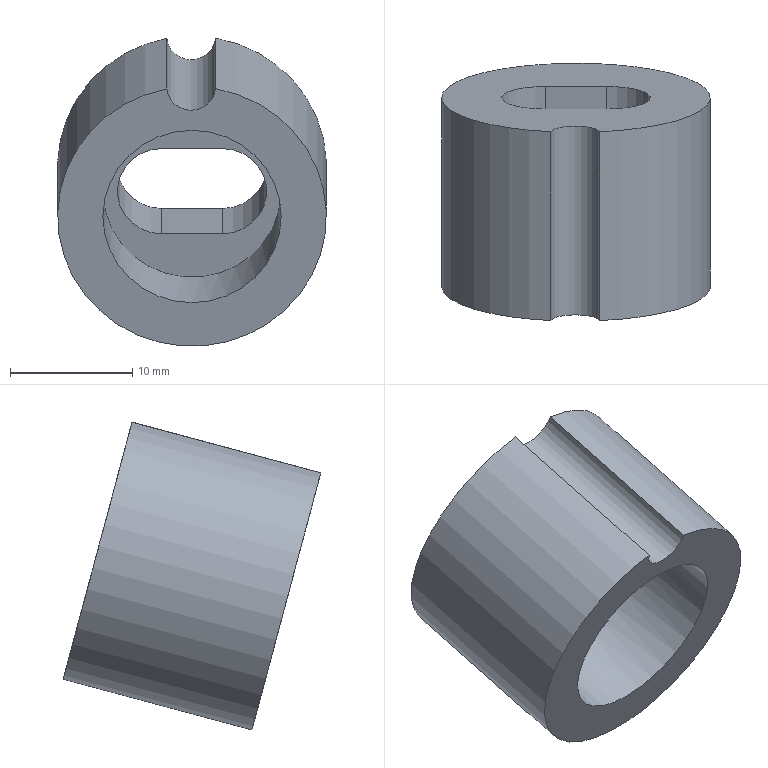Part | NX | features solid 2 | 1 solid | 10 faces | box 22 x 21.105 x 25.227 mm | volume 4030 mm3 | plane 5 | cylinder 5 | commonest cylinder face diameters 7.22 x2 4 x1 14.6 x1 22 x1
STEP:
#1=CARTESIAN_POINT('',(-406.307,59.873,-23.154));
#2=VERTEX_POINT('',#1);
#3=CARTESIAN_POINT('',(-402.324,59.867,-23.131));
#4=VERTEX_POINT('',#3);
#5=CARTESIAN_POINT('',(-404.316,59.823,-22.965));
#6=DIRECTION('',(0.,-0.9659,-0.2588));
#7=DIRECTION('',(0.999,0.01147,-0.04282));
#8=AXIS2_PLACEMENT_3D('',#5,#6,#7);
#9=CIRCLE('',#8,2.);
#10=EDGE_CURVE('',#2,#4,#9,.T.);
#11=ORIENTED_EDGE('',*,*,#10,.T.);
#12=CARTESIAN_POINT('',(-404.25,62.67,-33.592));
#13=DIRECTION('',(0.,0.9659,0.2588));
#14=DIRECTION('',(0.,-0.2588,0.9659));
#15=AXIS2_PLACEMENT_3D('',#12,#13,#14);
#16=CIRCLE('',#15,11.);
#17=EDGE_CURVE('',#2,#4,#16,.F.);
#18=ORIENTED_EDGE('',*,*,#17,.F.);
#19=EDGE_LOOP('',(#11,#18));
#20=FACE_BOUND('',#19,.T.);
#21=CARTESIAN_POINT('',(-401.75,63.604,-37.079));
#22=VERTEX_POINT('',#21);
#23=CARTESIAN_POINT('',(-401.75,61.736,-30.105));
#24=VERTEX_POINT('',#23);
#25=CARTESIAN_POINT('',(-401.75,62.67,-33.592));
#26=DIRECTION('',(0.,0.9659,0.2588));
#27=DIRECTION('',(0.,-0.2588,0.9659));
#28=AXIS2_PLACEMENT_3D('',#25,#26,#27);
#29=CIRCLE('',#28,3.61);
#30=EDGE_CURVE('',#22,#24,#29,.F.);
#31=ORIENTED_EDGE('',*,*,#30,.T.);
#32=CARTESIAN_POINT('',(-406.75,61.736,-30.105));
#33=VERTEX_POINT('',#32);
#34=CARTESIAN_POINT('',(-404.25,61.736,-30.105));
#35=DIRECTION('',(-1.,0.,0.));
#36=VECTOR('',#35,1000.);
#37=LINE('',#34,#36);
#38=EDGE_CURVE('',#24,#33,#37,.T.);
#39=ORIENTED_EDGE('',*,*,#38,.T.);
#40=CARTESIAN_POINT('',(-406.75,63.604,-37.079));
#41=VERTEX_POINT('',#40);
#42=CARTESIAN_POINT('',(-406.75,62.67,-33.592));
#43=DIRECTION('',(0.,0.9659,0.2588));
#44=DIRECTION('',(0.,-0.2588,0.9659));
#45=AXIS2_PLACEMENT_3D('',#42,#43,#44);
#46=CIRCLE('',#45,3.61);
#47=EDGE_CURVE('',#33,#41,#46,.F.);
#48=ORIENTED_EDGE('',*,*,#47,.T.);
#49=CARTESIAN_POINT('',(-404.25,63.604,-37.079));
#50=DIRECTION('',(1.,0.,0.));
#51=VECTOR('',#50,1000.);
#52=LINE('',#49,#51);
#53=EDGE_CURVE('',#41,#22,#52,.T.);
#54=ORIENTED_EDGE('',*,*,#53,.T.);
#55=EDGE_LOOP('',(#31,#39,#48,#54));
#56=FACE_BOUND('',#55,.T.);
#57=CARTESIAN_POINT('',(-404.25,62.67,-33.592));
#58=DIRECTION('',(0.,0.9659,0.2588));
#59=DIRECTION('',(-0.999,-0.01147,0.04282));
#60=AXIS2_PLACEMENT_3D('',#57,#58,#59);
#61=PLANE('',#60);
#62=ADVANCED_FACE('',(#20,#56),#61,.T.);
#63=CARTESIAN_POINT('',(-402.324,44.412,-27.272));
#64=VERTEX_POINT('',#63);
#65=CARTESIAN_POINT('',(-406.307,44.418,-27.295));
#66=VERTEX_POINT('',#65);
#67=CARTESIAN_POINT('',(-404.316,44.368,-27.106));
#68=DIRECTION('',(0.,-0.9659,-0.2588));
#69=DIRECTION('',(0.,0.2588,-0.9659));
#70=AXIS2_PLACEMENT_3D('',#67,#68,#69);
#71=CIRCLE('',#70,2.);
#72=EDGE_CURVE('',#64,#66,#71,.F.);
#73=ORIENTED_EDGE('',*,*,#72,.T.);
#74=CARTESIAN_POINT('',(-404.25,47.215,-37.733));
#75=DIRECTION('',(0.,-0.9659,-0.2588));
#76=DIRECTION('',(0.,0.2588,-0.9659));
#77=AXIS2_PLACEMENT_3D('',#74,#75,#76);
#78=CIRCLE('',#77,11.);
#79=EDGE_CURVE('',#64,#66,#78,.F.);
#80=ORIENTED_EDGE('',*,*,#79,.F.);
#81=EDGE_LOOP('',(#73,#80));
#82=FACE_BOUND('',#81,.T.);
#83=CARTESIAN_POINT('',(-404.25,49.105,-44.784));
#84=VERTEX_POINT('',#83);
#85=CARTESIAN_POINT('',(-404.25,47.215,-37.733));
#86=DIRECTION('',(0.,-0.9659,-0.2588));
#87=DIRECTION('',(0.,0.2588,-0.9659));
#88=AXIS2_PLACEMENT_3D('',#85,#86,#87);
#89=CIRCLE('',#88,7.3);
#90=EDGE_CURVE('',#84,#84,#89,.F.);
#91=ORIENTED_EDGE('',*,*,#90,.T.);
#92=EDGE_LOOP('',(#91));
#93=FACE_BOUND('',#92,.T.);
#94=CARTESIAN_POINT('',(-404.25,47.215,-37.733));
#95=DIRECTION('',(0.,-0.9659,-0.2588));
#96=DIRECTION('',(0.999,0.01147,-0.04282));
#97=AXIS2_PLACEMENT_3D('',#94,#95,#96);
#98=PLANE('',#97);
#99=ADVANCED_FACE('',(#82,#93),#98,.T.);
#100=CARTESIAN_POINT('',(-402.324,52.14,-25.201));
#101=DIRECTION('',(0.,0.9659,0.2588));
#102=VECTOR('',#101,1000.);
#103=LINE('',#100,#102);
#104=EDGE_CURVE('',#64,#4,#103,.T.);
#105=ORIENTED_EDGE('',*,*,#104,.F.);
#106=ORIENTED_EDGE('',*,*,#79,.T.);
#107=CARTESIAN_POINT('',(-406.307,52.146,-25.225));
#108=DIRECTION('',(0.,0.9659,0.2588));
#109=VECTOR('',#108,1000.);
#110=LINE('',#107,#109);
#111=EDGE_CURVE('',#2,#66,#110,.F.);
#112=ORIENTED_EDGE('',*,*,#111,.F.);
#113=ORIENTED_EDGE('',*,*,#17,.T.);
#114=EDGE_LOOP('',(#105,#106,#112,#113));
#115=FACE_BOUND('',#114,.T.);
#116=CARTESIAN_POINT('',(-404.25,43.351,-38.768));
#117=DIRECTION('',(0.,0.9659,0.2588));
#118=DIRECTION('',(-0.999,-0.01147,0.04282));
#119=AXIS2_PLACEMENT_3D('',#116,#117,#118);
#120=CYLINDRICAL_SURFACE('',#119,11.);
#121=ADVANCED_FACE('',(#115),#120,.T.);
#122=CARTESIAN_POINT('',(-406.75,54.008,-32.176));
#123=VERTEX_POINT('',#122);
#124=CARTESIAN_POINT('',(-401.75,54.008,-32.176));
#125=VERTEX_POINT('',#124);
#126=CARTESIAN_POINT('',(-404.25,54.008,-32.176));
#127=DIRECTION('',(1.,0.,0.));
#128=VECTOR('',#127,1000.);
#129=LINE('',#126,#128);
#130=EDGE_CURVE('',#123,#125,#129,.T.);
#131=ORIENTED_EDGE('',*,*,#130,.T.);
#132=CARTESIAN_POINT('',(-401.75,55.877,-39.15));
#133=VERTEX_POINT('',#132);
#134=CARTESIAN_POINT('',(-401.75,54.943,-35.663));
#135=DIRECTION('',(0.,0.9659,0.2588));
#136=DIRECTION('',(0.,-0.2588,0.9659));
#137=AXIS2_PLACEMENT_3D('',#134,#135,#136);
#138=CIRCLE('',#137,3.61);
#139=EDGE_CURVE('',#125,#133,#138,.T.);
#140=ORIENTED_EDGE('',*,*,#139,.T.);
#141=CARTESIAN_POINT('',(-406.75,55.877,-39.15));
#142=VERTEX_POINT('',#141);
#143=CARTESIAN_POINT('',(-404.25,55.877,-39.15));
#144=DIRECTION('',(-1.,0.,0.));
#145=VECTOR('',#144,1000.);
#146=LINE('',#143,#145);
#147=EDGE_CURVE('',#133,#142,#146,.T.);
#148=ORIENTED_EDGE('',*,*,#147,.T.);
#149=CARTESIAN_POINT('',(-406.75,54.943,-35.663));
#150=DIRECTION('',(0.,0.9659,0.2588));
#151=DIRECTION('',(0.,-0.2588,0.9659));
#152=AXIS2_PLACEMENT_3D('',#149,#150,#151);
#153=CIRCLE('',#152,3.61);
#154=EDGE_CURVE('',#142,#123,#153,.T.);
#155=ORIENTED_EDGE('',*,*,#154,.T.);
#156=EDGE_LOOP('',(#131,#140,#148,#155));
#157=FACE_BOUND('',#156,.T.);
#158=CARTESIAN_POINT('',(-404.25,53.053,-28.611));
#159=VERTEX_POINT('',#158);
#160=CARTESIAN_POINT('',(-404.25,54.943,-35.663));
#161=DIRECTION('',(0.,0.9659,0.2588));
#162=DIRECTION('',(0.,-0.2588,0.9659));
#163=AXIS2_PLACEMENT_3D('',#160,#161,#162);
#164=CIRCLE('',#163,7.3);
#165=EDGE_CURVE('',#159,#159,#164,.F.);
#166=ORIENTED_EDGE('',*,*,#165,.T.);
#167=EDGE_LOOP('',(#166));
#168=FACE_BOUND('',#167,.T.);
#169=CARTESIAN_POINT('',(-404.25,54.943,-35.663));
#170=DIRECTION('',(0.,0.9659,0.2588));
#171=DIRECTION('',(-0.999,-0.01147,0.04282));
#172=AXIS2_PLACEMENT_3D('',#169,#170,#171);
#173=PLANE('',#172);
#174=ADVANCED_FACE('',(#157,#168),#173,.F.);
#175=ORIENTED_EDGE('',*,*,#165,.F.);
#176=EDGE_LOOP('',(#175));
#177=FACE_BOUND('',#176,.T.);
#178=ORIENTED_EDGE('',*,*,#90,.F.);
#179=EDGE_LOOP('',(#178));
#180=FACE_BOUND('',#179,.T.);
#181=CARTESIAN_POINT('',(-404.25,43.351,-38.768));
#182=DIRECTION('',(0.,0.9659,0.2588));
#183=DIRECTION('',(-0.999,-0.01147,0.04282));
#184=AXIS2_PLACEMENT_3D('',#181,#182,#183);
#185=CYLINDRICAL_SURFACE('',#184,7.3);
#186=ADVANCED_FACE('',(#177,#180),#185,.F.);
#187=CARTESIAN_POINT('',(-406.75,55.877,-39.15));
#188=DIRECTION('',(0.,0.9659,0.2588));
#189=VECTOR('',#188,1000.);
#190=LINE('',#187,#189);
#191=EDGE_CURVE('',#142,#41,#190,.T.);
#192=ORIENTED_EDGE('',*,*,#191,.F.);
#193=ORIENTED_EDGE('',*,*,#147,.F.);
#194=CARTESIAN_POINT('',(-401.75,55.877,-39.15));
#195=DIRECTION('',(0.,0.9659,0.2588));
#196=VECTOR('',#195,1000.);
#197=LINE('',#194,#196);
#198=EDGE_CURVE('',#133,#22,#197,.T.);
#199=ORIENTED_EDGE('',*,*,#198,.T.);
#200=ORIENTED_EDGE('',*,*,#53,.F.);
#201=EDGE_LOOP('',(#192,#193,#199,#200));
#202=FACE_BOUND('',#201,.T.);
#203=CARTESIAN_POINT('',(-404.25,55.877,-39.15));
#204=DIRECTION('',(0.,0.2588,-0.9659));
#205=DIRECTION('',(0.,0.9659,0.2588));
#206=AXIS2_PLACEMENT_3D('',#203,#204,#205);
#207=PLANE('',#206);
#208=ADVANCED_FACE('',(#202),#207,.F.);
#209=ORIENTED_EDGE('',*,*,#130,.F.);
#210=CARTESIAN_POINT('',(-406.75,54.008,-32.176));
#211=DIRECTION('',(0.,-0.9659,-0.2588));
#212=VECTOR('',#211,1000.);
#213=LINE('',#210,#212);
#214=EDGE_CURVE('',#123,#33,#213,.F.);
#215=ORIENTED_EDGE('',*,*,#214,.T.);
#216=ORIENTED_EDGE('',*,*,#38,.F.);
#217=CARTESIAN_POINT('',(-401.75,54.008,-32.176));
#218=DIRECTION('',(0.,0.9659,0.2588));
#219=VECTOR('',#218,1000.);
#220=LINE('',#217,#219);
#221=EDGE_CURVE('',#125,#24,#220,.T.);
#222=ORIENTED_EDGE('',*,*,#221,.F.);
#223=EDGE_LOOP('',(#209,#215,#216,#222));
#224=FACE_BOUND('',#223,.T.);
#225=CARTESIAN_POINT('',(-404.25,54.008,-32.176));
#226=DIRECTION('',(0.,-0.2588,0.9659));
#227=DIRECTION('',(0.,-0.9659,-0.2588));
#228=AXIS2_PLACEMENT_3D('',#225,#226,#227);
#229=PLANE('',#228);
#230=ADVANCED_FACE('',(#224),#229,.F.);
#231=ORIENTED_EDGE('',*,*,#191,.T.);
#232=ORIENTED_EDGE('',*,*,#47,.F.);
#233=ORIENTED_EDGE('',*,*,#214,.F.);
#234=ORIENTED_EDGE('',*,*,#154,.F.);
#235=EDGE_LOOP('',(#231,#232,#233,#234));
#236=FACE_BOUND('',#235,.T.);
#237=CARTESIAN_POINT('',(-406.75,54.943,-35.663));
#238=DIRECTION('',(0.,0.9659,0.2588));
#239=DIRECTION('',(-0.999,-0.01147,0.04282));
#240=AXIS2_PLACEMENT_3D('',#237,#238,#239);
#241=CYLINDRICAL_SURFACE('',#240,3.61);
#242=ADVANCED_FACE('',(#236),#241,.F.);
#243=ORIENTED_EDGE('',*,*,#139,.F.);
#244=ORIENTED_EDGE('',*,*,#221,.T.);
#245=ORIENTED_EDGE('',*,*,#30,.F.);
#246=ORIENTED_EDGE('',*,*,#198,.F.);
#247=EDGE_LOOP('',(#243,#244,#245,#246));
#248=FACE_BOUND('',#247,.T.);
#249=CARTESIAN_POINT('',(-401.75,54.943,-35.663));
#250=DIRECTION('',(0.,0.9659,0.2588));
#251=DIRECTION('',(-0.999,-0.01147,0.04282));
#252=AXIS2_PLACEMENT_3D('',#249,#250,#251);
#253=CYLINDRICAL_SURFACE('',#252,3.61);
#254=ADVANCED_FACE('',(#248),#253,.F.);
#255=ORIENTED_EDGE('',*,*,#104,.T.);
#256=ORIENTED_EDGE('',*,*,#10,.F.);
#257=ORIENTED_EDGE('',*,*,#111,.T.);
#258=ORIENTED_EDGE('',*,*,#72,.F.);
#259=EDGE_LOOP('',(#255,#256,#257,#258));
#260=FACE_BOUND('',#259,.T.);
#261=CARTESIAN_POINT('',(-404.316,40.504,-28.142));
#262=DIRECTION('',(0.,0.9659,0.2588));
#263=DIRECTION('',(-0.999,-0.01147,0.04282));
#264=AXIS2_PLACEMENT_3D('',#261,#262,#263);
#265=CYLINDRICAL_SURFACE('',#264,2.);
#266=ADVANCED_FACE('',(#260),#265,.F.);
#267=CLOSED_SHELL('',(#62,#99,#121,#174,#186,#208,#230,#242,#254,#266));
#268=MANIFOLD_SOLID_BREP('',#267);
#269=(LENGTH_UNIT()NAMED_UNIT(*)SI_UNIT(.MILLI.,.METRE.));
#270=UNCERTAINTY_MEASURE_WITH_UNIT(LENGTH_MEASURE(0.00001),#269,'','');
#271=(NAMED_UNIT(*)PLANE_ANGLE_UNIT()SI_UNIT($,.RADIAN.));
#272=(NAMED_UNIT(*)SI_UNIT($,.STERADIAN.)SOLID_ANGLE_UNIT());
#273=(GEOMETRIC_REPRESENTATION_CONTEXT(3)GLOBAL_UNCERTAINTY_ASSIGNED_CONTEXT((#270))GLOBAL_UNIT_ASSIGNED_CONTEXT((#269,#271,#272))REPRESENTATION_CONTEXT('',''));
#274=ADVANCED_BREP_SHAPE_REPRESENTATION('',(#268),#273);